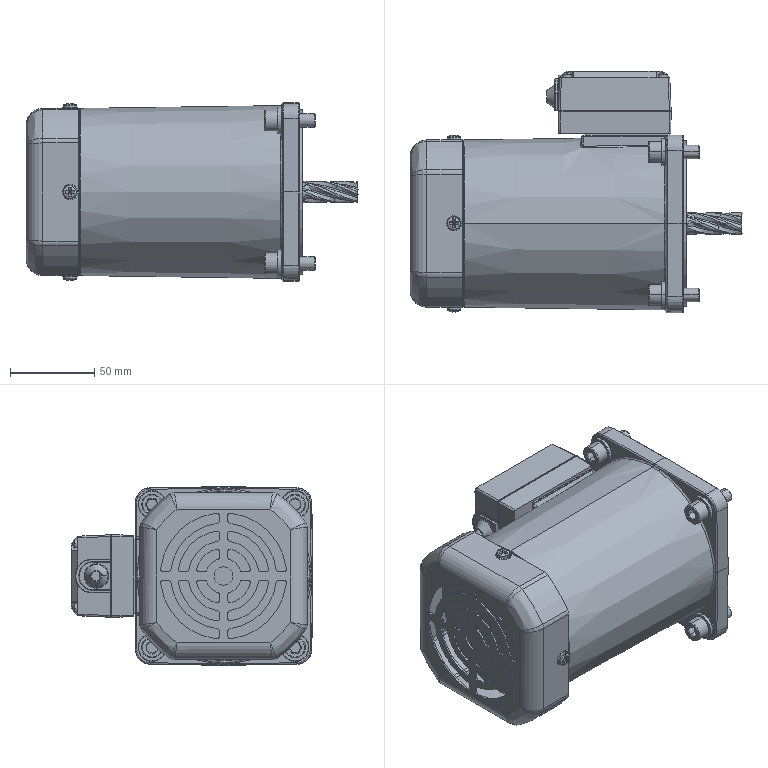Part | SolidWorks | features BaseBody 6 | 6 solids | 2571 faces | box 197 x 143.386 x 105.972 mm | volume 432731 mm3 | plane 1398 | cylinder 602 | spline 490 | cone 67 | torus 14 | commonest cylinder face diameters 2 x81 3 x59 4 x50 5 x42 0.5 x40 1 x38